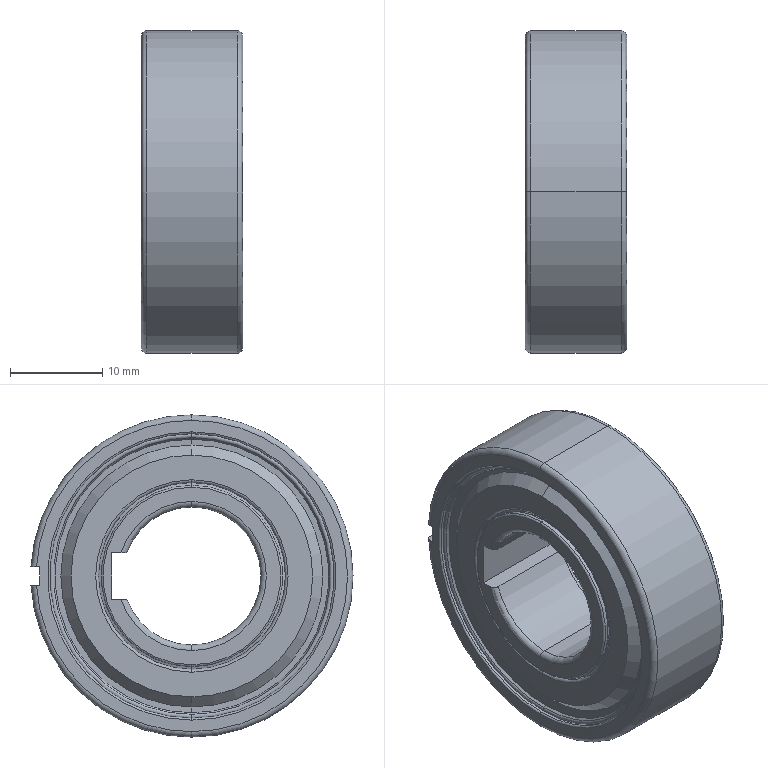Part | STEP file | BAY6202ZZ-J^One-way housed bearing | 1 solid | 144 faces | box 11 x 34.971 x 35 mm | volume 6760 mm3 | torus 52 | cone 40 | cylinder 34 | plane 18 | commonest cylinder face diameters 18.8 x4 19.7 x4 20.3 x4 20.9 x4 21.1 x4 28.9 x4